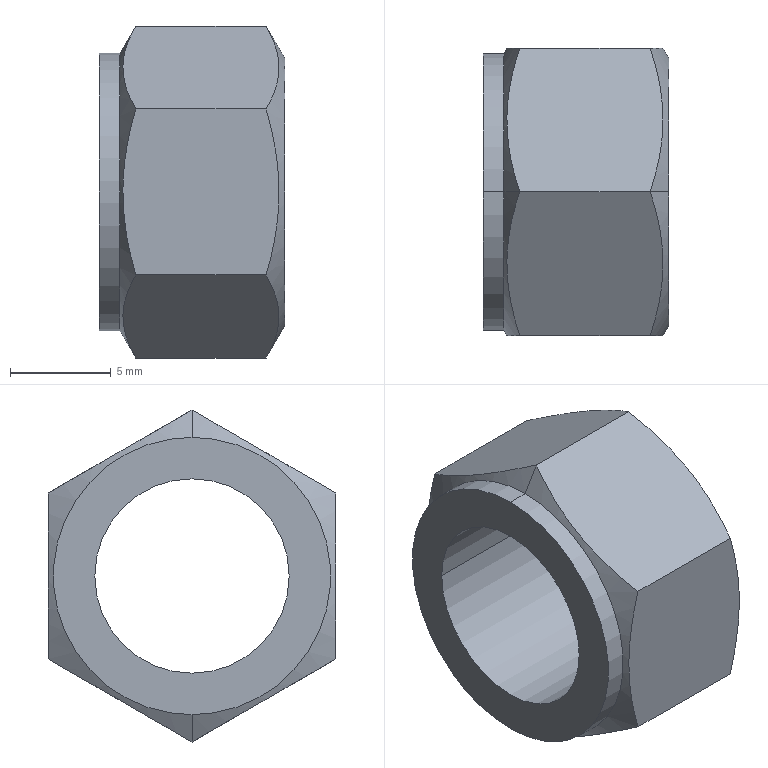Part | NX | features BREP 1 | 1 solid | 16 faces | box 9.22 x 14.275 x 16.483 mm | volume 906.398 mm3 | plane 8 | cylinder 4 | cone 4 | commonest cylinder face diameters 9.652 x2 13.767 x2
STEP:
#1=CARTESIAN_POINT('',(8.331,0.,6.634));
#2=VERTEX_POINT('',#1);
#3=CARTESIAN_POINT('',(8.331,0.,-6.634));
#4=VERTEX_POINT('',#3);
#5=CARTESIAN_POINT('',(8.331,0.,0.));
#6=DIRECTION('',(-1.,0.,0.));
#7=DIRECTION('',(0.,0.,1.));
#8=AXIS2_PLACEMENT_3D('',#5,#6,#7);
#9=CIRCLE('',#8,6.634);
#10=EDGE_CURVE('',#2,#4,#9,.T.);
#11=ORIENTED_EDGE('',*,*,#10,.F.);
#12=CARTESIAN_POINT('',(8.331,0.,0.));
#13=DIRECTION('',(-1.,0.,0.));
#14=DIRECTION('',(0.,0.,-1.));
#15=AXIS2_PLACEMENT_3D('',#12,#13,#14);
#16=CIRCLE('',#15,6.634);
#17=EDGE_CURVE('',#4,#2,#16,.T.);
#18=ORIENTED_EDGE('',*,*,#17,.F.);
#19=EDGE_LOOP('',(#11,#18));
#20=FACE_BOUND('',#19,.T.);
#21=CARTESIAN_POINT('',(8.331,-4.826,0.));
#22=VERTEX_POINT('',#21);
#23=CARTESIAN_POINT('',(8.331,4.826,0.));
#24=VERTEX_POINT('',#23);
#25=CARTESIAN_POINT('',(8.331,0.,0.));
#26=DIRECTION('',(1.,0.,0.));
#27=DIRECTION('',(0.,-1.,0.));
#28=AXIS2_PLACEMENT_3D('',#25,#26,#27);
#29=CIRCLE('',#28,4.826);
#30=EDGE_CURVE('',#22,#24,#29,.T.);
#31=ORIENTED_EDGE('',*,*,#30,.F.);
#32=CARTESIAN_POINT('',(8.331,0.,0.));
#33=DIRECTION('',(1.,0.,0.));
#34=DIRECTION('',(0.,1.,0.));
#35=AXIS2_PLACEMENT_3D('',#32,#33,#34);
#36=CIRCLE('',#35,4.826);
#37=EDGE_CURVE('',#24,#22,#36,.T.);
#38=ORIENTED_EDGE('',*,*,#37,.F.);
#39=EDGE_LOOP('',(#31,#38));
#40=FACE_BOUND('',#39,.T.);
#41=CARTESIAN_POINT('',(8.331,0.,0.));
#42=DIRECTION('',(1.,0.,0.));
#43=DIRECTION('',(0.,1.,0.));
#44=AXIS2_PLACEMENT_3D('',#41,#42,#43);
#45=PLANE('',#44);
#46=ADVANCED_FACE('',(#20,#40),#45,.T.);
#47=ORIENTED_EDGE('',*,*,#37,.T.);
#48=CARTESIAN_POINT('',(-0.889,-4.826,0.));
#49=VERTEX_POINT('',#48);
#50=CARTESIAN_POINT('',(-0.889,-4.826,0.));
#51=DIRECTION('',(1.,0.,0.));
#52=VECTOR('',#51,1000.);
#53=LINE('',#50,#52);
#54=EDGE_CURVE('',#22,#49,#53,.F.);
#55=ORIENTED_EDGE('',*,*,#54,.T.);
#56=CARTESIAN_POINT('',(-0.889,4.826,0.));
#57=VERTEX_POINT('',#56);
#58=CARTESIAN_POINT('',(-0.889,0.,0.));
#59=DIRECTION('',(1.,0.,0.));
#60=DIRECTION('',(0.,1.,0.));
#61=AXIS2_PLACEMENT_3D('',#58,#59,#60);
#62=CIRCLE('',#61,4.826);
#63=EDGE_CURVE('',#57,#49,#62,.T.);
#64=ORIENTED_EDGE('',*,*,#63,.F.);
#65=CARTESIAN_POINT('',(-0.889,4.826,0.));
#66=DIRECTION('',(1.,0.,0.));
#67=VECTOR('',#66,1000.);
#68=LINE('',#65,#67);
#69=EDGE_CURVE('',#24,#57,#68,.F.);
#70=ORIENTED_EDGE('',*,*,#69,.F.);
#71=EDGE_LOOP('',(#47,#55,#64,#70));
#72=FACE_BOUND('',#71,.T.);
#73=CARTESIAN_POINT('',(-1.811,0.,0.));
#74=DIRECTION('',(1.,0.,0.));
#75=DIRECTION('',(0.,1.,0.));
#76=AXIS2_PLACEMENT_3D('',#73,#74,#75);
#77=CYLINDRICAL_SURFACE('',#76,4.826);
#78=ADVANCED_FACE('',(#72),#77,.F.);
#79=CARTESIAN_POINT('',(-0.889,0.,0.));
#80=DIRECTION('',(1.,0.,0.));
#81=DIRECTION('',(0.,-1.,0.));
#82=AXIS2_PLACEMENT_3D('',#79,#80,#81);
#83=CIRCLE('',#82,4.826);
#84=EDGE_CURVE('',#49,#57,#83,.T.);
#85=ORIENTED_EDGE('',*,*,#84,.F.);
#86=ORIENTED_EDGE('',*,*,#54,.F.);
#87=ORIENTED_EDGE('',*,*,#30,.T.);
#88=ORIENTED_EDGE('',*,*,#69,.T.);
#89=EDGE_LOOP('',(#85,#86,#87,#88));
#90=FACE_BOUND('',#89,.T.);
#91=CARTESIAN_POINT('',(-1.811,0.,0.));
#92=DIRECTION('',(1.,0.,0.));
#93=DIRECTION('',(0.,1.,0.));
#94=AXIS2_PLACEMENT_3D('',#91,#92,#93);
#95=CYLINDRICAL_SURFACE('',#94,4.826);
#96=ADVANCED_FACE('',(#90),#95,.F.);
#97=CARTESIAN_POINT('',(-0.889,0.,6.883));
#98=VERTEX_POINT('',#97);
#99=CARTESIAN_POINT('',(-0.889,0.,-6.883));
#100=VERTEX_POINT('',#99);
#101=CARTESIAN_POINT('',(-0.889,0.,0.));
#102=DIRECTION('',(-1.,0.,0.));
#103=DIRECTION('',(0.,0.,1.));
#104=AXIS2_PLACEMENT_3D('',#101,#102,#103);
#105=CIRCLE('',#104,6.883);
#106=EDGE_CURVE('',#98,#100,#105,.T.);
#107=ORIENTED_EDGE('',*,*,#106,.T.);
#108=CARTESIAN_POINT('',(-0.889,0.,0.));
#109=DIRECTION('',(-1.,0.,0.));
#110=DIRECTION('',(0.,0.,-1.));
#111=AXIS2_PLACEMENT_3D('',#108,#109,#110);
#112=CIRCLE('',#111,6.883);
#113=EDGE_CURVE('',#100,#98,#112,.T.);
#114=ORIENTED_EDGE('',*,*,#113,.T.);
#115=EDGE_LOOP('',(#107,#114));
#116=FACE_BOUND('',#115,.T.);
#117=ORIENTED_EDGE('',*,*,#84,.T.);
#118=ORIENTED_EDGE('',*,*,#63,.T.);
#119=EDGE_LOOP('',(#117,#118));
#120=FACE_BOUND('',#119,.T.);
#121=CARTESIAN_POINT('',(-0.889,0.,0.));
#122=DIRECTION('',(-1.,0.,0.));
#123=DIRECTION('',(0.,0.,1.));
#124=AXIS2_PLACEMENT_3D('',#121,#122,#123);
#125=PLANE('',#124);
#126=ADVANCED_FACE('',(#116,#120),#125,.T.);
#127=CARTESIAN_POINT('',(0.1437,0.,6.883));
#128=VERTEX_POINT('',#127);
#129=CARTESIAN_POINT('',(0.1437,0.,6.883));
#130=DIRECTION('',(-1.,0.,0.));
#131=VECTOR('',#130,1000.);
#132=LINE('',#129,#131);
#133=EDGE_CURVE('',#98,#128,#132,.F.);
#134=ORIENTED_EDGE('',*,*,#133,.F.);
#135=ORIENTED_EDGE('',*,*,#113,.F.);
#136=CARTESIAN_POINT('',(0.1437,0.,-6.883));
#137=VERTEX_POINT('',#136);
#138=CARTESIAN_POINT('',(0.1437,0.,-6.883));
#139=DIRECTION('',(-1.,0.,0.));
#140=VECTOR('',#139,1000.);
#141=LINE('',#138,#140);
#142=EDGE_CURVE('',#100,#137,#141,.F.);
#143=ORIENTED_EDGE('',*,*,#142,.T.);
#144=CARTESIAN_POINT('',(0.1437,0.,0.));
#145=DIRECTION('',(-1.,0.,0.));
#146=DIRECTION('',(0.,0.,-1.));
#147=AXIS2_PLACEMENT_3D('',#144,#145,#146);
#148=CIRCLE('',#147,6.883);
#149=EDGE_CURVE('',#137,#128,#148,.T.);
#150=ORIENTED_EDGE('',*,*,#149,.T.);
#151=EDGE_LOOP('',(#134,#135,#143,#150));
#152=FACE_BOUND('',#151,.T.);
#153=CARTESIAN_POINT('',(0.508,0.,0.));
#154=DIRECTION('',(-1.,0.,0.));
#155=DIRECTION('',(0.,0.,-1.));
#156=AXIS2_PLACEMENT_3D('',#153,#154,#155);
#157=CYLINDRICAL_SURFACE('',#156,6.883);
#158=ADVANCED_FACE('',(#152),#157,.T.);
#159=CARTESIAN_POINT('',(0.9279,0.,-8.242));
#160=VERTEX_POINT('',#159);
#161=CARTESIAN_POINT('',(0.1437,0.,-6.883));
#162=DIRECTION('',(0.5,0.,-0.866));
#163=VECTOR('',#162,1000.);
#164=LINE('',#161,#163);
#165=EDGE_CURVE('',#137,#160,#164,.T.);
#166=ORIENTED_EDGE('',*,*,#165,.T.);
#167=CARTESIAN_POINT('',(0.9279,-7.137,-4.121));
#168=VERTEX_POINT('',#167);
#169=CARTESIAN_POINT('',(0.9279,-7.137,-4.121));
#170=CARTESIAN_POINT('',(0.07885,-4.59,-5.591));
#171=CARTESIAN_POINT('',(0.07821,-2.549,-6.77));
#172=CARTESIAN_POINT('',(0.9279,0.,-8.242));
#173=B_SPLINE_CURVE_WITH_KNOTS('',3,(#169,#170,#171,#172),.UNSPECIFIED.,.F.,.F.,(4,4),(0.,1.),.UNSPECIFIED.);
#174=EDGE_CURVE('',#160,#168,#173,.F.);
#175=ORIENTED_EDGE('',*,*,#174,.T.);
#176=CARTESIAN_POINT('',(0.9279,-7.137,4.121));
#177=VERTEX_POINT('',#176);
#178=CARTESIAN_POINT('',(0.9279,-7.137,4.121));
#179=CARTESIAN_POINT('',(0.07885,-7.137,1.18));
#180=CARTESIAN_POINT('',(0.07821,-7.137,-1.178));
#181=CARTESIAN_POINT('',(0.9279,-7.137,-4.121));
#182=B_SPLINE_CURVE_WITH_KNOTS('',3,(#178,#179,#180,#181),.UNSPECIFIED.,.F.,.F.,(4,4),(0.,1.),.UNSPECIFIED.);
#183=EDGE_CURVE('',#168,#177,#182,.F.);
#184=ORIENTED_EDGE('',*,*,#183,.T.);
#185=CARTESIAN_POINT('',(0.9279,0.,8.242));
#186=VERTEX_POINT('',#185);
#187=CARTESIAN_POINT('',(0.9279,0.,8.242));
#188=CARTESIAN_POINT('',(0.07885,-2.547,6.771));
#189=CARTESIAN_POINT('',(0.07821,-4.588,5.592));
#190=CARTESIAN_POINT('',(0.9279,-7.137,4.121));
#191=B_SPLINE_CURVE_WITH_KNOTS('',3,(#187,#188,#189,#190),.UNSPECIFIED.,.F.,.F.,(4,4),(0.,1.),.UNSPECIFIED.);
#192=EDGE_CURVE('',#177,#186,#191,.F.);
#193=ORIENTED_EDGE('',*,*,#192,.T.);
#194=CARTESIAN_POINT('',(0.1437,0.,6.883));
#195=DIRECTION('',(0.5,0.,0.866));
#196=VECTOR('',#195,1000.);
#197=LINE('',#194,#196);
#198=EDGE_CURVE('',#128,#186,#197,.T.);
#199=ORIENTED_EDGE('',*,*,#198,.F.);
#200=ORIENTED_EDGE('',*,*,#149,.F.);
#201=EDGE_LOOP('',(#166,#175,#184,#193,#199,#200));
#202=FACE_BOUND('',#201,.T.);
#203=CARTESIAN_POINT('',(0.5358,0.,0.));
#204=DIRECTION('',(1.,0.,0.));
#205=DIRECTION('',(0.,0.,1.));
#206=AXIS2_PLACEMENT_3D('',#203,#204,#205);
#207=CONICAL_SURFACE('',#206,7.562,1.047);
#208=ADVANCED_FACE('',(#202),#207,.T.);
#209=ORIENTED_EDGE('',*,*,#198,.T.);
#210=CARTESIAN_POINT('',(0.9279,7.137,4.121));
#211=VERTEX_POINT('',#210);
#212=CARTESIAN_POINT('',(0.9279,7.137,4.121));
#213=CARTESIAN_POINT('',(0.07885,4.59,5.591));
#214=CARTESIAN_POINT('',(0.07821,2.549,6.77));
#215=CARTESIAN_POINT('',(0.9279,0.,8.242));
#216=B_SPLINE_CURVE_WITH_KNOTS('',3,(#212,#213,#214,#215),.UNSPECIFIED.,.F.,.F.,(4,4),(0.,1.),.UNSPECIFIED.);
#217=EDGE_CURVE('',#186,#211,#216,.F.);
#218=ORIENTED_EDGE('',*,*,#217,.T.);
#219=CARTESIAN_POINT('',(0.9279,7.137,-4.121));
#220=VERTEX_POINT('',#219);
#221=CARTESIAN_POINT('',(0.9279,7.137,-4.121));
#222=CARTESIAN_POINT('',(0.07885,7.137,-1.18));
#223=CARTESIAN_POINT('',(0.07821,7.137,1.178));
#224=CARTESIAN_POINT('',(0.9279,7.137,4.121));
#225=B_SPLINE_CURVE_WITH_KNOTS('',3,(#221,#222,#223,#224),.UNSPECIFIED.,.F.,.F.,(4,4),(0.,1.),.UNSPECIFIED.);
#226=EDGE_CURVE('',#211,#220,#225,.F.);
#227=ORIENTED_EDGE('',*,*,#226,.T.);
#228=CARTESIAN_POINT('',(0.9279,0.,-8.242));
#229=CARTESIAN_POINT('',(0.07885,2.547,-6.771));
#230=CARTESIAN_POINT('',(0.07821,4.588,-5.592));
#231=CARTESIAN_POINT('',(0.9279,7.137,-4.121));
#232=B_SPLINE_CURVE_WITH_KNOTS('',3,(#228,#229,#230,#231),.UNSPECIFIED.,.F.,.F.,(4,4),(0.,1.),.UNSPECIFIED.);
#233=EDGE_CURVE('',#220,#160,#232,.F.);
#234=ORIENTED_EDGE('',*,*,#233,.T.);
#235=ORIENTED_EDGE('',*,*,#165,.F.);
#236=CARTESIAN_POINT('',(0.1437,0.,0.));
#237=DIRECTION('',(-1.,0.,0.));
#238=DIRECTION('',(0.,0.,1.));
#239=AXIS2_PLACEMENT_3D('',#236,#237,#238);
#240=CIRCLE('',#239,6.883);
#241=EDGE_CURVE('',#128,#137,#240,.T.);
#242=ORIENTED_EDGE('',*,*,#241,.F.);
#243=EDGE_LOOP('',(#209,#218,#227,#234,#235,#242));
#244=FACE_BOUND('',#243,.T.);
#245=CARTESIAN_POINT('',(0.5358,0.,0.));
#246=DIRECTION('',(1.,0.,0.));
#247=DIRECTION('',(0.,0.,1.));
#248=AXIS2_PLACEMENT_3D('',#245,#246,#247);
#249=CONICAL_SURFACE('',#248,7.562,1.047);
#250=ADVANCED_FACE('',(#244),#249,.T.);
#251=ORIENTED_EDGE('',*,*,#142,.F.);
#252=ORIENTED_EDGE('',*,*,#106,.F.);
#253=ORIENTED_EDGE('',*,*,#133,.T.);
#254=ORIENTED_EDGE('',*,*,#241,.T.);
#255=EDGE_LOOP('',(#251,#252,#253,#254));
#256=FACE_BOUND('',#255,.T.);
#257=CARTESIAN_POINT('',(0.508,0.,0.));
#258=DIRECTION('',(-1.,0.,0.));
#259=DIRECTION('',(0.,0.,-1.));
#260=AXIS2_PLACEMENT_3D('',#257,#258,#259);
#261=CYLINDRICAL_SURFACE('',#260,6.883);
#262=ADVANCED_FACE('',(#256),#261,.T.);
#263=CARTESIAN_POINT('',(7.403,0.,-8.242));
#264=VERTEX_POINT('',#263);
#265=CARTESIAN_POINT('',(0.9279,0.,-8.242));
#266=DIRECTION('',(1.,0.,0.));
#267=VECTOR('',#266,1000.);
#268=LINE('',#265,#267);
#269=EDGE_CURVE('',#160,#264,#268,.T.);
#270=ORIENTED_EDGE('',*,*,#269,.F.);
#271=ORIENTED_EDGE('',*,*,#233,.F.);
#272=CARTESIAN_POINT('',(7.403,7.137,-4.121));
#273=VERTEX_POINT('',#272);
#274=CARTESIAN_POINT('',(0.9279,7.137,-4.121));
#275=DIRECTION('',(1.,0.,0.));
#276=VECTOR('',#275,1000.);
#277=LINE('',#274,#276);
#278=EDGE_CURVE('',#220,#273,#277,.T.);
#279=ORIENTED_EDGE('',*,*,#278,.T.);
#280=CARTESIAN_POINT('',(7.403,7.137,-4.121));
#281=CARTESIAN_POINT('',(8.252,4.59,-5.591));
#282=CARTESIAN_POINT('',(8.253,2.549,-6.77));
#283=CARTESIAN_POINT('',(7.403,0.,-8.242));
#284=B_SPLINE_CURVE_WITH_KNOTS('',3,(#280,#281,#282,#283),.UNSPECIFIED.,.F.,.F.,(4,4),(0.,1.),.UNSPECIFIED.);
#285=EDGE_CURVE('',#273,#264,#284,.T.);
#286=ORIENTED_EDGE('',*,*,#285,.T.);
#287=EDGE_LOOP('',(#270,#271,#279,#286));
#288=FACE_BOUND('',#287,.T.);
#289=CARTESIAN_POINT('',(0.,0.,-8.242));
#290=DIRECTION('',(0.,0.5,-0.866));
#291=DIRECTION('',(-1.,0.,0.));
#292=AXIS2_PLACEMENT_3D('',#289,#290,#291);
#293=PLANE('',#292);
#294=ADVANCED_FACE('',(#288),#293,.T.);
#295=CARTESIAN_POINT('',(8.331,0.,-6.634));
#296=DIRECTION('',(-0.5,0.,-0.866));
#297=VECTOR('',#296,1000.);
#298=LINE('',#295,#297);
#299=EDGE_CURVE('',#4,#264,#298,.T.);
#300=ORIENTED_EDGE('',*,*,#299,.T.);
#301=ORIENTED_EDGE('',*,*,#285,.F.);
#302=CARTESIAN_POINT('',(7.403,7.137,4.121));
#303=VERTEX_POINT('',#302);
#304=CARTESIAN_POINT('',(7.403,7.137,4.121));
#305=CARTESIAN_POINT('',(8.252,7.137,1.18));
#306=CARTESIAN_POINT('',(8.253,7.137,-1.177));
#307=CARTESIAN_POINT('',(7.403,7.137,-4.121));
#308=B_SPLINE_CURVE_WITH_KNOTS('',3,(#304,#305,#306,#307),.UNSPECIFIED.,.F.,.F.,(4,4),(0.,1.),.UNSPECIFIED.);
#309=EDGE_CURVE('',#303,#273,#308,.T.);
#310=ORIENTED_EDGE('',*,*,#309,.F.);
#311=CARTESIAN_POINT('',(7.403,0.,8.242));
#312=VERTEX_POINT('',#311);
#313=CARTESIAN_POINT('',(7.403,0.,8.242));
#314=CARTESIAN_POINT('',(8.252,2.547,6.771));
#315=CARTESIAN_POINT('',(8.253,4.588,5.593));
#316=CARTESIAN_POINT('',(7.403,7.137,4.121));
#317=B_SPLINE_CURVE_WITH_KNOTS('',3,(#313,#314,#315,#316),.UNSPECIFIED.,.F.,.F.,(4,4),(0.,1.),.UNSPECIFIED.);
#318=EDGE_CURVE('',#312,#303,#317,.T.);
#319=ORIENTED_EDGE('',*,*,#318,.F.);
#320=CARTESIAN_POINT('',(8.331,0.,6.634));
#321=DIRECTION('',(-0.5,0.,0.866));
#322=VECTOR('',#321,1000.);
#323=LINE('',#320,#322);
#324=EDGE_CURVE('',#2,#312,#323,.T.);
#325=ORIENTED_EDGE('',*,*,#324,.F.);
#326=ORIENTED_EDGE('',*,*,#10,.T.);
#327=EDGE_LOOP('',(#300,#301,#310,#319,#325,#326));
#328=FACE_BOUND('',#327,.T.);
#329=CARTESIAN_POINT('',(7.867,0.,0.));
#330=DIRECTION('',(-1.,0.,0.));
#331=DIRECTION('',(0.,0.,-1.));
#332=AXIS2_PLACEMENT_3D('',#329,#330,#331);
#333=CONICAL_SURFACE('',#332,7.438,1.047);
#334=ADVANCED_FACE('',(#328),#333,.T.);
#335=ORIENTED_EDGE('',*,*,#324,.T.);
#336=CARTESIAN_POINT('',(7.403,-7.137,4.121));
#337=VERTEX_POINT('',#336);
#338=CARTESIAN_POINT('',(7.403,-7.137,4.121));
#339=CARTESIAN_POINT('',(8.252,-4.59,5.591));
#340=CARTESIAN_POINT('',(8.253,-2.549,6.77));
#341=CARTESIAN_POINT('',(7.403,0.,8.242));
#342=B_SPLINE_CURVE_WITH_KNOTS('',3,(#338,#339,#340,#341),.UNSPECIFIED.,.F.,.F.,(4,4),(0.,1.),.UNSPECIFIED.);
#343=EDGE_CURVE('',#337,#312,#342,.T.);
#344=ORIENTED_EDGE('',*,*,#343,.F.);
#345=CARTESIAN_POINT('',(7.403,-7.137,-4.121));
#346=VERTEX_POINT('',#345);
#347=CARTESIAN_POINT('',(7.403,-7.137,-4.121));
#348=CARTESIAN_POINT('',(8.252,-7.137,-1.18));
#349=CARTESIAN_POINT('',(8.253,-7.137,1.177));
#350=CARTESIAN_POINT('',(7.403,-7.137,4.121));
#351=B_SPLINE_CURVE_WITH_KNOTS('',3,(#347,#348,#349,#350),.UNSPECIFIED.,.F.,.F.,(4,4),(0.,1.),.UNSPECIFIED.);
#352=EDGE_CURVE('',#346,#337,#351,.T.);
#353=ORIENTED_EDGE('',*,*,#352,.F.);
#354=CARTESIAN_POINT('',(7.403,0.,-8.242));
#355=CARTESIAN_POINT('',(8.252,-2.547,-6.771));
#356=CARTESIAN_POINT('',(8.253,-4.588,-5.593));
#357=CARTESIAN_POINT('',(7.403,-7.137,-4.121));
#358=B_SPLINE_CURVE_WITH_KNOTS('',3,(#354,#355,#356,#357),.UNSPECIFIED.,.F.,.F.,(4,4),(0.,1.),.UNSPECIFIED.);
#359=EDGE_CURVE('',#264,#346,#358,.T.);
#360=ORIENTED_EDGE('',*,*,#359,.F.);
#361=ORIENTED_EDGE('',*,*,#299,.F.);
#362=ORIENTED_EDGE('',*,*,#17,.T.);
#363=EDGE_LOOP('',(#335,#344,#353,#360,#361,#362));
#364=FACE_BOUND('',#363,.T.);
#365=CARTESIAN_POINT('',(7.867,0.,0.));
#366=DIRECTION('',(-1.,0.,0.));
#367=DIRECTION('',(0.,0.,-1.));
#368=AXIS2_PLACEMENT_3D('',#365,#366,#367);
#369=CONICAL_SURFACE('',#368,7.438,1.047);
#370=ADVANCED_FACE('',(#364),#369,.T.);
#371=CARTESIAN_POINT('',(0.9279,-7.137,-4.121));
#372=DIRECTION('',(1.,0.,0.));
#373=VECTOR('',#372,1000.);
#374=LINE('',#371,#373);
#375=EDGE_CURVE('',#168,#346,#374,.T.);
#376=ORIENTED_EDGE('',*,*,#375,.F.);
#377=ORIENTED_EDGE('',*,*,#174,.F.);
#378=ORIENTED_EDGE('',*,*,#269,.T.);
#379=ORIENTED_EDGE('',*,*,#359,.T.);
#380=EDGE_LOOP('',(#376,#377,#378,#379));
#381=FACE_BOUND('',#380,.T.);
#382=CARTESIAN_POINT('',(0.,-7.137,-4.121));
#383=DIRECTION('',(0.,-0.5,-0.866));
#384=DIRECTION('',(0.,-0.866,0.5));
#385=AXIS2_PLACEMENT_3D('',#382,#383,#384);
#386=PLANE('',#385);
#387=ADVANCED_FACE('',(#381),#386,.T.);
#388=CARTESIAN_POINT('',(0.9279,-7.137,4.121));
#389=DIRECTION('',(1.,0.,0.));
#390=VECTOR('',#389,1000.);
#391=LINE('',#388,#390);
#392=EDGE_CURVE('',#177,#337,#391,.T.);
#393=ORIENTED_EDGE('',*,*,#392,.F.);
#394=ORIENTED_EDGE('',*,*,#183,.F.);
#395=ORIENTED_EDGE('',*,*,#375,.T.);
#396=ORIENTED_EDGE('',*,*,#352,.T.);
#397=EDGE_LOOP('',(#393,#394,#395,#396));
#398=FACE_BOUND('',#397,.T.);
#399=CARTESIAN_POINT('',(0.,-7.137,4.121));
#400=DIRECTION('',(0.,-1.,0.));
#401=DIRECTION('',(0.,0.,-1.));
#402=AXIS2_PLACEMENT_3D('',#399,#400,#401);
#403=PLANE('',#402);
#404=ADVANCED_FACE('',(#398),#403,.T.);
#405=CARTESIAN_POINT('',(0.9279,0.,8.242));
#406=DIRECTION('',(1.,0.,0.));
#407=VECTOR('',#406,1000.);
#408=LINE('',#405,#407);
#409=EDGE_CURVE('',#186,#312,#408,.T.);
#410=ORIENTED_EDGE('',*,*,#409,.F.);
#411=ORIENTED_EDGE('',*,*,#192,.F.);
#412=ORIENTED_EDGE('',*,*,#392,.T.);
#413=ORIENTED_EDGE('',*,*,#343,.T.);
#414=EDGE_LOOP('',(#410,#411,#412,#413));
#415=FACE_BOUND('',#414,.T.);
#416=CARTESIAN_POINT('',(0.,0.,8.242));
#417=DIRECTION('',(0.,-0.5,0.866));
#418=DIRECTION('',(-1.,0.,0.));
#419=AXIS2_PLACEMENT_3D('',#416,#417,#418);
#420=PLANE('',#419);
#421=ADVANCED_FACE('',(#415),#420,.T.);
#422=CARTESIAN_POINT('',(0.9279,7.137,4.121));
#423=DIRECTION('',(1.,0.,0.));
#424=VECTOR('',#423,1000.);
#425=LINE('',#422,#424);
#426=EDGE_CURVE('',#211,#303,#425,.T.);
#427=ORIENTED_EDGE('',*,*,#426,.F.);
#428=ORIENTED_EDGE('',*,*,#217,.F.);
#429=ORIENTED_EDGE('',*,*,#409,.T.);
#430=ORIENTED_EDGE('',*,*,#318,.T.);
#431=EDGE_LOOP('',(#427,#428,#429,#430));
#432=FACE_BOUND('',#431,.T.);
#433=CARTESIAN_POINT('',(0.,7.137,4.121));
#434=DIRECTION('',(0.,0.5,0.866));
#435=DIRECTION('',(1.,0.,0.));
#436=AXIS2_PLACEMENT_3D('',#433,#434,#435);
#437=PLANE('',#436);
#438=ADVANCED_FACE('',(#432),#437,.T.);
#439=ORIENTED_EDGE('',*,*,#278,.F.);
#440=ORIENTED_EDGE('',*,*,#226,.F.);
#441=ORIENTED_EDGE('',*,*,#426,.T.);
#442=ORIENTED_EDGE('',*,*,#309,.T.);
#443=EDGE_LOOP('',(#439,#440,#441,#442));
#444=FACE_BOUND('',#443,.T.);
#445=CARTESIAN_POINT('',(0.,7.137,-4.121));
#446=DIRECTION('',(0.,1.,0.));
#447=DIRECTION('',(1.,0.,0.));
#448=AXIS2_PLACEMENT_3D('',#445,#446,#447);
#449=PLANE('',#448);
#450=ADVANCED_FACE('',(#444),#449,.T.);
#451=CLOSED_SHELL('',(#46,#78,#96,#126,#158,#208,#250,#262,#294,#334,#370,#387,#404,#421,#438,#450));
#452=MANIFOLD_SOLID_BREP('',#451);
#453=(LENGTH_UNIT()NAMED_UNIT(*)SI_UNIT(.MILLI.,.METRE.));
#454=UNCERTAINTY_MEASURE_WITH_UNIT(LENGTH_MEASURE(0.0508),#453,'','');
#455=(NAMED_UNIT(*)PLANE_ANGLE_UNIT()SI_UNIT($,.RADIAN.));
#456=(NAMED_UNIT(*)SI_UNIT($,.STERADIAN.)SOLID_ANGLE_UNIT());
#457=(GEOMETRIC_REPRESENTATION_CONTEXT(3)GLOBAL_UNCERTAINTY_ASSIGNED_CONTEXT((#454))GLOBAL_UNIT_ASSIGNED_CONTEXT((#453,#455,#456))REPRESENTATION_CONTEXT('',''));
#458=ADVANCED_BREP_SHAPE_REPRESENTATION('',(#452),#457);